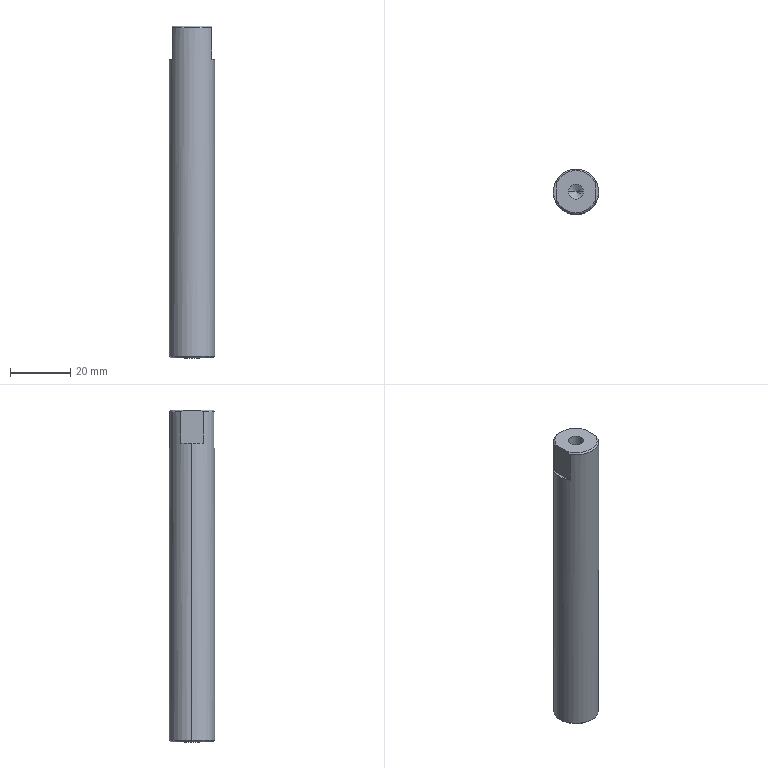Part | SolidWorks | features HoleWzd 2, BaseBody 1 | 1 solid | 20 faces | box 15 x 15 x 110 mm | volume 18709 mm3 | cone 8 | cylinder 6 | plane 6 | commonest cylinder face diameters 5 x4 15 x2
STEP:
#1=CARTESIAN_POINT('',(2.5,0.,-95.));
#2=VERTEX_POINT('',#1);
#3=CARTESIAN_POINT('',(-2.5,0.,-95.));
#4=VERTEX_POINT('',#3);
#5=CARTESIAN_POINT('',(0.,0.,-95.));
#6=DIRECTION('',(0.,0.,-1.));
#7=DIRECTION('',(-1.,0.,0.));
#8=AXIS2_PLACEMENT_3D('',#5,#6,#7);
#9=CIRCLE('',#8,2.5);
#10=EDGE_CURVE('',#2,#4,#9,.T.);
#11=ORIENTED_EDGE('',*,*,#10,.F.);
#12=CARTESIAN_POINT('',(2.5,0.,-110.));
#13=VERTEX_POINT('',#12);
#14=CARTESIAN_POINT('',(2.5,0.,-110.));
#15=DIRECTION('',(0.,0.,-1.));
#16=VECTOR('',#15,1000.);
#17=LINE('',#14,#16);
#18=EDGE_CURVE('',#2,#13,#17,.T.);
#19=ORIENTED_EDGE('',*,*,#18,.T.);
#20=CARTESIAN_POINT('',(-2.5,0.,-110.));
#21=VERTEX_POINT('',#20);
#22=CARTESIAN_POINT('',(0.,0.,-110.));
#23=DIRECTION('',(0.,0.,-1.));
#24=DIRECTION('',(-1.,0.,0.));
#25=AXIS2_PLACEMENT_3D('',#22,#23,#24);
#26=CIRCLE('',#25,2.5);
#27=EDGE_CURVE('',#13,#21,#26,.T.);
#28=ORIENTED_EDGE('',*,*,#27,.T.);
#29=CARTESIAN_POINT('',(-2.5,0.,-110.));
#30=DIRECTION('',(0.,0.,-1.));
#31=VECTOR('',#30,1000.);
#32=LINE('',#29,#31);
#33=EDGE_CURVE('',#4,#21,#32,.T.);
#34=ORIENTED_EDGE('',*,*,#33,.F.);
#35=EDGE_LOOP('',(#11,#19,#28,#34));
#36=FACE_OUTER_BOUND('',#35,.T.);
#37=CARTESIAN_POINT('',(0.,0.,-110.));
#38=DIRECTION('',(0.,0.,-1.));
#39=DIRECTION('',(-1.,0.,0.));
#40=AXIS2_PLACEMENT_3D('',#37,#38,#39);
#41=CYLINDRICAL_SURFACE('',#40,2.5);
#42=ADVANCED_FACE('',(#36),#41,.F.);
#43=CARTESIAN_POINT('',(0.,0.,-93.498));
#44=VERTEX_POINT('',#43);
#45=CARTESIAN_POINT('',(-2.5,0.,-95.));
#46=DIRECTION('',(-0.8572,0.,-0.515));
#47=VECTOR('',#46,1000.);
#48=LINE('',#45,#47);
#49=EDGE_CURVE('',#44,#4,#48,.T.);
#50=ORIENTED_EDGE('',*,*,#49,.F.);
#51=CARTESIAN_POINT('',(2.5,0.,-95.));
#52=DIRECTION('',(0.8572,0.,-0.515));
#53=VECTOR('',#52,1000.);
#54=LINE('',#51,#53);
#55=EDGE_CURVE('',#44,#2,#54,.T.);
#56=ORIENTED_EDGE('',*,*,#55,.T.);
#57=ORIENTED_EDGE('',*,*,#10,.T.);
#58=EDGE_LOOP('',(#50,#56,#57));
#59=FACE_OUTER_BOUND('',#58,.T.);
#60=CARTESIAN_POINT('',(0.,0.,-95.));
#61=DIRECTION('',(0.,0.,-1.));
#62=DIRECTION('',(-1.,0.,0.));
#63=AXIS2_PLACEMENT_3D('',#60,#61,#62);
#64=CONICAL_SURFACE('',#63,2.5,1.03);
#65=ADVANCED_FACE('',(#59),#64,.F.);
#66=CARTESIAN_POINT('',(-2.5,0.,-15.));
#67=VERTEX_POINT('',#66);
#68=CARTESIAN_POINT('',(2.5,0.,-15.));
#69=VERTEX_POINT('',#68);
#70=CARTESIAN_POINT('',(0.,0.,-15.));
#71=DIRECTION('',(0.,0.,1.));
#72=DIRECTION('',(1.,0.,0.));
#73=AXIS2_PLACEMENT_3D('',#70,#71,#72);
#74=CIRCLE('',#73,2.5);
#75=EDGE_CURVE('',#67,#69,#74,.T.);
#76=ORIENTED_EDGE('',*,*,#75,.F.);
#77=CARTESIAN_POINT('',(-2.5,0.,0.));
#78=VERTEX_POINT('',#77);
#79=CARTESIAN_POINT('',(-2.5,0.,0.));
#80=DIRECTION('',(0.,0.,1.));
#81=VECTOR('',#80,1000.);
#82=LINE('',#79,#81);
#83=EDGE_CURVE('',#67,#78,#82,.T.);
#84=ORIENTED_EDGE('',*,*,#83,.T.);
#85=CARTESIAN_POINT('',(2.5,0.,0.));
#86=VERTEX_POINT('',#85);
#87=CARTESIAN_POINT('',(0.,0.,0.));
#88=DIRECTION('',(0.,0.,1.));
#89=DIRECTION('',(1.,0.,0.));
#90=AXIS2_PLACEMENT_3D('',#87,#88,#89);
#91=CIRCLE('',#90,2.5);
#92=EDGE_CURVE('',#78,#86,#91,.T.);
#93=ORIENTED_EDGE('',*,*,#92,.T.);
#94=CARTESIAN_POINT('',(2.5,0.,0.));
#95=DIRECTION('',(0.,0.,1.));
#96=VECTOR('',#95,1000.);
#97=LINE('',#94,#96);
#98=EDGE_CURVE('',#69,#86,#97,.T.);
#99=ORIENTED_EDGE('',*,*,#98,.F.);
#100=EDGE_LOOP('',(#76,#84,#93,#99));
#101=FACE_OUTER_BOUND('',#100,.T.);
#102=CARTESIAN_POINT('',(0.,0.,0.));
#103=DIRECTION('',(0.,0.,1.));
#104=DIRECTION('',(1.,0.,0.));
#105=AXIS2_PLACEMENT_3D('',#102,#103,#104);
#106=CYLINDRICAL_SURFACE('',#105,2.5);
#107=ADVANCED_FACE('',(#101),#106,.F.);
#108=CARTESIAN_POINT('',(0.,0.,-16.502));
#109=VERTEX_POINT('',#108);
#110=CARTESIAN_POINT('',(2.5,0.,-15.));
#111=DIRECTION('',(0.8572,0.,0.515));
#112=VECTOR('',#111,1000.);
#113=LINE('',#110,#112);
#114=EDGE_CURVE('',#109,#69,#113,.T.);
#115=ORIENTED_EDGE('',*,*,#114,.F.);
#116=CARTESIAN_POINT('',(-2.5,0.,-15.));
#117=DIRECTION('',(-0.8572,0.,0.515));
#118=VECTOR('',#117,1000.);
#119=LINE('',#116,#118);
#120=EDGE_CURVE('',#109,#67,#119,.T.);
#121=ORIENTED_EDGE('',*,*,#120,.T.);
#122=ORIENTED_EDGE('',*,*,#75,.T.);
#123=EDGE_LOOP('',(#115,#121,#122));
#124=FACE_OUTER_BOUND('',#123,.T.);
#125=CARTESIAN_POINT('',(0.,0.,-15.));
#126=DIRECTION('',(0.,0.,1.));
#127=DIRECTION('',(1.,0.,0.));
#128=AXIS2_PLACEMENT_3D('',#125,#126,#127);
#129=CONICAL_SURFACE('',#128,2.5,1.03);
#130=ADVANCED_FACE('',(#124),#129,.F.);
#131=CARTESIAN_POINT('',(0.,7.5,-109.5));
#132=VERTEX_POINT('',#131);
#133=CARTESIAN_POINT('',(-7.5,0.,-109.5));
#134=VERTEX_POINT('',#133);
#135=CARTESIAN_POINT('',(0.,0.,-109.5));
#136=DIRECTION('',(0.,0.,1.));
#137=DIRECTION('',(1.,0.,0.));
#138=AXIS2_PLACEMENT_3D('',#135,#136,#137);
#139=CIRCLE('',#138,7.5);
#140=EDGE_CURVE('',#132,#134,#139,.T.);
#141=ORIENTED_EDGE('',*,*,#140,.T.);
#142=CARTESIAN_POINT('',(-7.5,0.,-11.));
#143=VERTEX_POINT('',#142);
#144=CARTESIAN_POINT('',(-7.5,0.,-110.));
#145=DIRECTION('',(0.,0.,1.));
#146=VECTOR('',#145,1000.);
#147=LINE('',#144,#146);
#148=EDGE_CURVE('',#134,#143,#147,.T.);
#149=ORIENTED_EDGE('',*,*,#148,.T.);
#150=CARTESIAN_POINT('',(-6.5,3.742,-11.));
#151=VERTEX_POINT('',#150);
#152=CARTESIAN_POINT('',(0.,0.,-11.));
#153=DIRECTION('',(0.,0.,-1.));
#154=DIRECTION('',(1.,0.,0.));
#155=AXIS2_PLACEMENT_3D('',#152,#153,#154);
#156=CIRCLE('',#155,7.5);
#157=EDGE_CURVE('',#143,#151,#156,.T.);
#158=ORIENTED_EDGE('',*,*,#157,.T.);
#159=CARTESIAN_POINT('',(-6.5,3.742,-0.5));
#160=VERTEX_POINT('',#159);
#161=CARTESIAN_POINT('',(-6.5,3.742,-110.));
#162=DIRECTION('',(0.,0.,1.));
#163=VECTOR('',#162,1000.);
#164=LINE('',#161,#163);
#165=EDGE_CURVE('',#151,#160,#164,.T.);
#166=ORIENTED_EDGE('',*,*,#165,.T.);
#167=CARTESIAN_POINT('',(6.5,3.742,-0.5));
#168=VERTEX_POINT('',#167);
#169=CARTESIAN_POINT('',(0.,0.,-0.5));
#170=DIRECTION('',(0.,0.,-1.));
#171=DIRECTION('',(1.,0.,0.));
#172=AXIS2_PLACEMENT_3D('',#169,#170,#171);
#173=CIRCLE('',#172,7.5);
#174=EDGE_CURVE('',#160,#168,#173,.T.);
#175=ORIENTED_EDGE('',*,*,#174,.T.);
#176=CARTESIAN_POINT('',(6.5,3.742,-11.));
#177=VERTEX_POINT('',#176);
#178=CARTESIAN_POINT('',(6.5,3.742,-110.));
#179=DIRECTION('',(0.,0.,-1.));
#180=VECTOR('',#179,1000.);
#181=LINE('',#178,#180);
#182=EDGE_CURVE('',#168,#177,#181,.T.);
#183=ORIENTED_EDGE('',*,*,#182,.T.);
#184=CARTESIAN_POINT('',(7.5,0.,-11.));
#185=VERTEX_POINT('',#184);
#186=CARTESIAN_POINT('',(0.,0.,-11.));
#187=DIRECTION('',(0.,0.,-1.));
#188=DIRECTION('',(1.,0.,0.));
#189=AXIS2_PLACEMENT_3D('',#186,#187,#188);
#190=CIRCLE('',#189,7.5);
#191=EDGE_CURVE('',#177,#185,#190,.T.);
#192=ORIENTED_EDGE('',*,*,#191,.T.);
#193=CARTESIAN_POINT('',(7.5,0.,-109.5));
#194=VERTEX_POINT('',#193);
#195=CARTESIAN_POINT('',(7.5,0.,-110.));
#196=DIRECTION('',(0.,0.,1.));
#197=VECTOR('',#196,1000.);
#198=LINE('',#195,#197);
#199=EDGE_CURVE('',#194,#185,#198,.T.);
#200=ORIENTED_EDGE('',*,*,#199,.F.);
#201=CARTESIAN_POINT('',(0.,0.,-109.5));
#202=DIRECTION('',(0.,0.,1.));
#203=DIRECTION('',(1.,0.,0.));
#204=AXIS2_PLACEMENT_3D('',#201,#202,#203);
#205=CIRCLE('',#204,7.5);
#206=EDGE_CURVE('',#194,#132,#205,.T.);
#207=ORIENTED_EDGE('',*,*,#206,.T.);
#208=EDGE_LOOP('',(#141,#149,#158,#166,#175,#183,#192,#200,#207));
#209=FACE_OUTER_BOUND('',#208,.T.);
#210=CARTESIAN_POINT('',(0.,0.,-110.));
#211=DIRECTION('',(0.,0.,1.));
#212=DIRECTION('',(1.,0.,0.));
#213=AXIS2_PLACEMENT_3D('',#210,#211,#212);
#214=CYLINDRICAL_SURFACE('',#213,7.5);
#215=ADVANCED_FACE('',(#209),#214,.T.);
#216=CARTESIAN_POINT('',(0.,-7.,-110.));
#217=VERTEX_POINT('',#216);
#218=CARTESIAN_POINT('',(0.,7.,-110.));
#219=VERTEX_POINT('',#218);
#220=CARTESIAN_POINT('',(0.,0.,-110.));
#221=DIRECTION('',(0.,0.,1.));
#222=DIRECTION('',(0.,-1.,0.));
#223=AXIS2_PLACEMENT_3D('',#220,#221,#222);
#224=CIRCLE('',#223,7.);
#225=EDGE_CURVE('',#217,#219,#224,.T.);
#226=ORIENTED_EDGE('',*,*,#225,.T.);
#227=CARTESIAN_POINT('',(0.,7.5,-109.5));
#228=DIRECTION('',(0.,0.7071,0.7071));
#229=VECTOR('',#228,1000.);
#230=LINE('',#227,#229);
#231=EDGE_CURVE('',#219,#132,#230,.T.);
#232=ORIENTED_EDGE('',*,*,#231,.T.);
#233=ORIENTED_EDGE('',*,*,#206,.F.);
#234=CARTESIAN_POINT('',(0.,-7.5,-109.5));
#235=VERTEX_POINT('',#234);
#236=CARTESIAN_POINT('',(0.,0.,-109.5));
#237=DIRECTION('',(0.,0.,1.));
#238=DIRECTION('',(1.,0.,0.));
#239=AXIS2_PLACEMENT_3D('',#236,#237,#238);
#240=CIRCLE('',#239,7.5);
#241=EDGE_CURVE('',#235,#194,#240,.T.);
#242=ORIENTED_EDGE('',*,*,#241,.F.);
#243=CARTESIAN_POINT('',(0.,-7.5,-109.5));
#244=DIRECTION('',(0.,-0.7071,0.7071));
#245=VECTOR('',#244,1000.);
#246=LINE('',#243,#245);
#247=EDGE_CURVE('',#217,#235,#246,.T.);
#248=ORIENTED_EDGE('',*,*,#247,.F.);
#249=EDGE_LOOP('',(#226,#232,#233,#242,#248));
#250=FACE_OUTER_BOUND('',#249,.T.);
#251=CARTESIAN_POINT('',(0.,0.,-109.5));
#252=DIRECTION('',(0.,0.,1.));
#253=DIRECTION('',(0.,-1.,0.));
#254=AXIS2_PLACEMENT_3D('',#251,#252,#253);
#255=CONICAL_SURFACE('',#254,7.5,0.7854);
#256=ADVANCED_FACE('',(#250),#255,.T.);
#257=ORIENTED_EDGE('',*,*,#148,.F.);
#258=CARTESIAN_POINT('',(0.,0.,-109.5));
#259=DIRECTION('',(0.,0.,1.));
#260=DIRECTION('',(1.,0.,0.));
#261=AXIS2_PLACEMENT_3D('',#258,#259,#260);
#262=CIRCLE('',#261,7.5);
#263=EDGE_CURVE('',#134,#235,#262,.T.);
#264=ORIENTED_EDGE('',*,*,#263,.T.);
#265=ORIENTED_EDGE('',*,*,#241,.T.);
#266=ORIENTED_EDGE('',*,*,#199,.T.);
#267=CARTESIAN_POINT('',(6.5,-3.742,-11.));
#268=VERTEX_POINT('',#267);
#269=CARTESIAN_POINT('',(0.,0.,-11.));
#270=DIRECTION('',(0.,0.,-1.));
#271=DIRECTION('',(1.,0.,0.));
#272=AXIS2_PLACEMENT_3D('',#269,#270,#271);
#273=CIRCLE('',#272,7.5);
#274=EDGE_CURVE('',#185,#268,#273,.T.);
#275=ORIENTED_EDGE('',*,*,#274,.T.);
#276=CARTESIAN_POINT('',(6.5,-3.742,-0.5));
#277=VERTEX_POINT('',#276);
#278=CARTESIAN_POINT('',(6.5,-3.742,-110.));
#279=DIRECTION('',(0.,0.,1.));
#280=VECTOR('',#279,1000.);
#281=LINE('',#278,#280);
#282=EDGE_CURVE('',#268,#277,#281,.T.);
#283=ORIENTED_EDGE('',*,*,#282,.T.);
#284=CARTESIAN_POINT('',(-6.5,-3.742,-0.5));
#285=VERTEX_POINT('',#284);
#286=CARTESIAN_POINT('',(0.,0.,-0.5));
#287=DIRECTION('',(0.,0.,-1.));
#288=DIRECTION('',(1.,0.,0.));
#289=AXIS2_PLACEMENT_3D('',#286,#287,#288);
#290=CIRCLE('',#289,7.5);
#291=EDGE_CURVE('',#277,#285,#290,.T.);
#292=ORIENTED_EDGE('',*,*,#291,.T.);
#293=CARTESIAN_POINT('',(-6.5,-3.742,-11.));
#294=VERTEX_POINT('',#293);
#295=CARTESIAN_POINT('',(-6.5,-3.742,-110.));
#296=DIRECTION('',(0.,0.,-1.));
#297=VECTOR('',#296,1000.);
#298=LINE('',#295,#297);
#299=EDGE_CURVE('',#285,#294,#298,.T.);
#300=ORIENTED_EDGE('',*,*,#299,.T.);
#301=CARTESIAN_POINT('',(0.,0.,-11.));
#302=DIRECTION('',(0.,0.,-1.));
#303=DIRECTION('',(1.,0.,0.));
#304=AXIS2_PLACEMENT_3D('',#301,#302,#303);
#305=CIRCLE('',#304,7.5);
#306=EDGE_CURVE('',#294,#143,#305,.T.);
#307=ORIENTED_EDGE('',*,*,#306,.T.);
#308=EDGE_LOOP('',(#257,#264,#265,#266,#275,#283,#292,#300,#307));
#309=FACE_OUTER_BOUND('',#308,.T.);
#310=CARTESIAN_POINT('',(0.,0.,-110.));
#311=DIRECTION('',(0.,0.,1.));
#312=DIRECTION('',(1.,0.,0.));
#313=AXIS2_PLACEMENT_3D('',#310,#311,#312);
#314=CYLINDRICAL_SURFACE('',#313,7.5);
#315=ADVANCED_FACE('',(#309),#314,.T.);
#316=ORIENTED_EDGE('',*,*,#306,.F.);
#317=CARTESIAN_POINT('',(-6.5,0.,-11.));
#318=DIRECTION('',(0.,1.,0.));
#319=VECTOR('',#318,1000.);
#320=LINE('',#317,#319);
#321=EDGE_CURVE('',#294,#151,#320,.T.);
#322=ORIENTED_EDGE('',*,*,#321,.T.);
#323=ORIENTED_EDGE('',*,*,#157,.F.);
#324=EDGE_LOOP('',(#316,#322,#323));
#325=FACE_OUTER_BOUND('',#324,.T.);
#326=CARTESIAN_POINT('',(0.,0.,-11.));
#327=DIRECTION('',(0.,0.,1.));
#328=DIRECTION('',(1.,0.,0.));
#329=AXIS2_PLACEMENT_3D('',#326,#327,#328);
#330=PLANE('',#329);
#331=ADVANCED_FACE('',(#325),#330,.T.);
#332=ORIENTED_EDGE('',*,*,#321,.F.);
#333=ORIENTED_EDGE('',*,*,#299,.F.);
#334=CARTESIAN_POINT('',(-6.5,-2.598,0.));
#335=VERTEX_POINT('',#334);
#336=CARTESIAN_POINT('',(-6.5,-3.742,-0.5));
#337=CARTESIAN_POINT('',(-6.5,-3.369,-0.314));
#338=CARTESIAN_POINT('',(-6.5,-2.989,-0.145));
#339=CARTESIAN_POINT('',(-6.5,-2.598,0.));
#340=B_SPLINE_CURVE_WITH_KNOTS('',3,(#336,#337,#338,#339),.UNSPECIFIED.,.F.,.F.,(4,4),(0.,0.001248),.UNSPECIFIED.);
#341=EDGE_CURVE('',#285,#335,#340,.T.);
#342=ORIENTED_EDGE('',*,*,#341,.T.);
#343=CARTESIAN_POINT('',(-6.5,2.598,0.));
#344=VERTEX_POINT('',#343);
#345=CARTESIAN_POINT('',(-6.5,3.742,0.));
#346=DIRECTION('',(0.,1.,0.));
#347=VECTOR('',#346,1000.);
#348=LINE('',#345,#347);
#349=EDGE_CURVE('',#335,#344,#348,.T.);
#350=ORIENTED_EDGE('',*,*,#349,.T.);
#351=CARTESIAN_POINT('',(-6.5,2.598,0.));
#352=CARTESIAN_POINT('',(-6.5,2.989,-0.145));
#353=CARTESIAN_POINT('',(-6.5,3.369,-0.314));
#354=CARTESIAN_POINT('',(-6.5,3.742,-0.5));
#355=B_SPLINE_CURVE_WITH_KNOTS('',3,(#351,#352,#353,#354),.UNSPECIFIED.,.F.,.F.,(4,4),(0.,0.001248),.UNSPECIFIED.);
#356=EDGE_CURVE('',#344,#160,#355,.T.);
#357=ORIENTED_EDGE('',*,*,#356,.T.);
#358=ORIENTED_EDGE('',*,*,#165,.F.);
#359=EDGE_LOOP('',(#332,#333,#342,#350,#357,#358));
#360=FACE_OUTER_BOUND('',#359,.T.);
#361=CARTESIAN_POINT('',(-6.5,3.742,-11.));
#362=DIRECTION('',(-1.,0.,0.));
#363=DIRECTION('',(0.,0.,1.));
#364=AXIS2_PLACEMENT_3D('',#361,#362,#363);
#365=PLANE('',#364);
#366=ADVANCED_FACE('',(#360),#365,.T.);
#367=ORIENTED_EDGE('',*,*,#341,.F.);
#368=ORIENTED_EDGE('',*,*,#291,.F.);
#369=CARTESIAN_POINT('',(6.5,-2.598,0.));
#370=VERTEX_POINT('',#369);
#371=CARTESIAN_POINT('',(6.5,-3.742,-0.5));
#372=CARTESIAN_POINT('',(6.5,-3.369,-0.314));
#373=CARTESIAN_POINT('',(6.5,-2.989,-0.145));
#374=CARTESIAN_POINT('',(6.5,-2.598,0.));
#375=B_SPLINE_CURVE_WITH_KNOTS('',3,(#371,#372,#373,#374),.UNSPECIFIED.,.F.,.F.,(4,4),(0.,0.001248),.UNSPECIFIED.);
#376=EDGE_CURVE('',#277,#370,#375,.T.);
#377=ORIENTED_EDGE('',*,*,#376,.T.);
#378=CARTESIAN_POINT('',(0.,0.,0.));
#379=DIRECTION('',(0.,0.,-1.));
#380=DIRECTION('',(0.,1.,0.));
#381=AXIS2_PLACEMENT_3D('',#378,#379,#380);
#382=CIRCLE('',#381,7.);
#383=EDGE_CURVE('',#370,#335,#382,.T.);
#384=ORIENTED_EDGE('',*,*,#383,.T.);
#385=EDGE_LOOP('',(#367,#368,#377,#384));
#386=FACE_OUTER_BOUND('',#385,.T.);
#387=CARTESIAN_POINT('',(0.,0.,-0.5));
#388=DIRECTION('',(0.,0.,-1.));
#389=DIRECTION('',(0.,1.,0.));
#390=AXIS2_PLACEMENT_3D('',#387,#388,#389);
#391=CONICAL_SURFACE('',#390,7.5,0.7854);
#392=ADVANCED_FACE('',(#386),#391,.T.);
#393=CARTESIAN_POINT('',(6.5,-3.742,-11.));
#394=DIRECTION('',(0.,1.,0.));
#395=VECTOR('',#394,1000.);
#396=LINE('',#393,#395);
#397=EDGE_CURVE('',#268,#177,#396,.T.);
#398=ORIENTED_EDGE('',*,*,#397,.T.);
#399=ORIENTED_EDGE('',*,*,#182,.F.);
#400=CARTESIAN_POINT('',(6.5,2.598,0.));
#401=VERTEX_POINT('',#400);
#402=CARTESIAN_POINT('',(6.5,3.742,-0.5));
#403=CARTESIAN_POINT('',(6.5,3.369,-0.314));
#404=CARTESIAN_POINT('',(6.5,2.989,-0.145));
#405=CARTESIAN_POINT('',(6.5,2.598,0.));
#406=B_SPLINE_CURVE_WITH_KNOTS('',3,(#402,#403,#404,#405),.UNSPECIFIED.,.F.,.F.,(4,4),(0.,0.001248),.UNSPECIFIED.);
#407=EDGE_CURVE('',#168,#401,#406,.T.);
#408=ORIENTED_EDGE('',*,*,#407,.T.);
#409=CARTESIAN_POINT('',(6.5,-3.742,0.));
#410=DIRECTION('',(0.,-1.,0.));
#411=VECTOR('',#410,1000.);
#412=LINE('',#409,#411);
#413=EDGE_CURVE('',#401,#370,#412,.T.);
#414=ORIENTED_EDGE('',*,*,#413,.T.);
#415=ORIENTED_EDGE('',*,*,#376,.F.);
#416=ORIENTED_EDGE('',*,*,#282,.F.);
#417=EDGE_LOOP('',(#398,#399,#408,#414,#415,#416));
#418=FACE_OUTER_BOUND('',#417,.T.);
#419=CARTESIAN_POINT('',(6.5,-3.742,-11.));
#420=DIRECTION('',(1.,0.,0.));
#421=DIRECTION('',(0.,0.,-1.));
#422=AXIS2_PLACEMENT_3D('',#419,#420,#421);
#423=PLANE('',#422);
#424=ADVANCED_FACE('',(#418),#423,.T.);
#425=ORIENTED_EDGE('',*,*,#191,.F.);
#426=ORIENTED_EDGE('',*,*,#397,.F.);
#427=ORIENTED_EDGE('',*,*,#274,.F.);
#428=EDGE_LOOP('',(#425,#426,#427));
#429=FACE_OUTER_BOUND('',#428,.T.);
#430=CARTESIAN_POINT('',(0.,0.,-11.));
#431=DIRECTION('',(0.,0.,1.));
#432=DIRECTION('',(1.,0.,0.));
#433=AXIS2_PLACEMENT_3D('',#430,#431,#432);
#434=PLANE('',#433);
#435=ADVANCED_FACE('',(#429),#434,.T.);
#436=ORIENTED_EDGE('',*,*,#407,.F.);
#437=ORIENTED_EDGE('',*,*,#174,.F.);
#438=ORIENTED_EDGE('',*,*,#356,.F.);
#439=CARTESIAN_POINT('',(0.,0.,0.));
#440=DIRECTION('',(0.,0.,-1.));
#441=DIRECTION('',(-1.,0.,0.));
#442=AXIS2_PLACEMENT_3D('',#439,#440,#441);
#443=CIRCLE('',#442,7.);
#444=EDGE_CURVE('',#344,#401,#443,.T.);
#445=ORIENTED_EDGE('',*,*,#444,.T.);
#446=EDGE_LOOP('',(#436,#437,#438,#445));
#447=FACE_OUTER_BOUND('',#446,.T.);
#448=CARTESIAN_POINT('',(0.,0.,-0.5));
#449=DIRECTION('',(0.,0.,-1.));
#450=DIRECTION('',(-1.,0.,0.));
#451=AXIS2_PLACEMENT_3D('',#448,#449,#450);
#452=CONICAL_SURFACE('',#451,7.5,0.7854);
#453=ADVANCED_FACE('',(#447),#452,.T.);
#454=ORIENTED_EDGE('',*,*,#231,.F.);
#455=CARTESIAN_POINT('',(0.,0.,-110.));
#456=DIRECTION('',(0.,0.,1.));
#457=DIRECTION('',(0.,-1.,0.));
#458=AXIS2_PLACEMENT_3D('',#455,#456,#457);
#459=CIRCLE('',#458,7.);
#460=EDGE_CURVE('',#219,#217,#459,.T.);
#461=ORIENTED_EDGE('',*,*,#460,.T.);
#462=ORIENTED_EDGE('',*,*,#247,.T.);
#463=ORIENTED_EDGE('',*,*,#263,.F.);
#464=ORIENTED_EDGE('',*,*,#140,.F.);
#465=EDGE_LOOP('',(#454,#461,#462,#463,#464));
#466=FACE_OUTER_BOUND('',#465,.T.);
#467=CARTESIAN_POINT('',(0.,0.,-109.5));
#468=DIRECTION('',(0.,0.,1.));
#469=DIRECTION('',(0.,-1.,0.));
#470=AXIS2_PLACEMENT_3D('',#467,#468,#469);
#471=CONICAL_SURFACE('',#470,7.5,0.7854);
#472=ADVANCED_FACE('',(#466),#471,.T.);
#473=CARTESIAN_POINT('',(0.,0.,0.));
#474=DIRECTION('',(0.,0.,1.));
#475=DIRECTION('',(1.,0.,0.));
#476=AXIS2_PLACEMENT_3D('',#473,#474,#475);
#477=CIRCLE('',#476,2.5);
#478=EDGE_CURVE('',#86,#78,#477,.T.);
#479=ORIENTED_EDGE('',*,*,#478,.F.);
#480=ORIENTED_EDGE('',*,*,#92,.F.);
#481=EDGE_LOOP('',(#479,#480));
#482=FACE_BOUND('',#481,.T.);
#483=ORIENTED_EDGE('',*,*,#349,.F.);
#484=ORIENTED_EDGE('',*,*,#383,.F.);
#485=ORIENTED_EDGE('',*,*,#413,.F.);
#486=ORIENTED_EDGE('',*,*,#444,.F.);
#487=EDGE_LOOP('',(#483,#484,#485,#486));
#488=FACE_OUTER_BOUND('',#487,.T.);
#489=CARTESIAN_POINT('',(0.,0.,0.));
#490=DIRECTION('',(0.,0.,-1.));
#491=DIRECTION('',(-1.,0.,0.));
#492=AXIS2_PLACEMENT_3D('',#489,#490,#491);
#493=PLANE('',#492);
#494=ADVANCED_FACE('',(#482,#488),#493,.F.);
#495=ORIENTED_EDGE('',*,*,#225,.F.);
#496=ORIENTED_EDGE('',*,*,#460,.F.);
#497=EDGE_LOOP('',(#495,#496));
#498=FACE_OUTER_BOUND('',#497,.T.);
#499=CARTESIAN_POINT('',(0.,0.,-110.));
#500=DIRECTION('',(0.,0.,-1.));
#501=DIRECTION('',(-1.,0.,0.));
#502=AXIS2_PLACEMENT_3D('',#499,#500,#501);
#503=CIRCLE('',#502,2.5);
#504=EDGE_CURVE('',#21,#13,#503,.T.);
#505=ORIENTED_EDGE('',*,*,#504,.F.);
#506=ORIENTED_EDGE('',*,*,#27,.F.);
#507=EDGE_LOOP('',(#505,#506));
#508=FACE_BOUND('',#507,.T.);
#509=CARTESIAN_POINT('',(0.,7.,-110.));
#510=DIRECTION('',(0.,0.,1.));
#511=DIRECTION('',(1.,0.,0.));
#512=AXIS2_PLACEMENT_3D('',#509,#510,#511);
#513=PLANE('',#512);
#514=ADVANCED_FACE('',(#498,#508),#513,.F.);
#515=ORIENTED_EDGE('',*,*,#120,.F.);
#516=ORIENTED_EDGE('',*,*,#114,.T.);
#517=CARTESIAN_POINT('',(0.,0.,-15.));
#518=DIRECTION('',(0.,0.,1.));
#519=DIRECTION('',(1.,0.,0.));
#520=AXIS2_PLACEMENT_3D('',#517,#518,#519);
#521=CIRCLE('',#520,2.5);
#522=EDGE_CURVE('',#69,#67,#521,.T.);
#523=ORIENTED_EDGE('',*,*,#522,.T.);
#524=EDGE_LOOP('',(#515,#516,#523));
#525=FACE_OUTER_BOUND('',#524,.T.);
#526=CARTESIAN_POINT('',(0.,0.,-15.));
#527=DIRECTION('',(0.,0.,1.));
#528=DIRECTION('',(1.,0.,0.));
#529=AXIS2_PLACEMENT_3D('',#526,#527,#528);
#530=CONICAL_SURFACE('',#529,2.5,1.03);
#531=ADVANCED_FACE('',(#525),#530,.F.);
#532=ORIENTED_EDGE('',*,*,#83,.F.);
#533=ORIENTED_EDGE('',*,*,#522,.F.);
#534=ORIENTED_EDGE('',*,*,#98,.T.);
#535=ORIENTED_EDGE('',*,*,#478,.T.);
#536=EDGE_LOOP('',(#532,#533,#534,#535));
#537=FACE_OUTER_BOUND('',#536,.T.);
#538=CARTESIAN_POINT('',(0.,0.,0.));
#539=DIRECTION('',(0.,0.,1.));
#540=DIRECTION('',(1.,0.,0.));
#541=AXIS2_PLACEMENT_3D('',#538,#539,#540);
#542=CYLINDRICAL_SURFACE('',#541,2.5);
#543=ADVANCED_FACE('',(#537),#542,.F.);
#544=ORIENTED_EDGE('',*,*,#55,.F.);
#545=ORIENTED_EDGE('',*,*,#49,.T.);
#546=CARTESIAN_POINT('',(0.,0.,-95.));
#547=DIRECTION('',(0.,0.,-1.));
#548=DIRECTION('',(-1.,0.,0.));
#549=AXIS2_PLACEMENT_3D('',#546,#547,#548);
#550=CIRCLE('',#549,2.5);
#551=EDGE_CURVE('',#4,#2,#550,.T.);
#552=ORIENTED_EDGE('',*,*,#551,.T.);
#553=EDGE_LOOP('',(#544,#545,#552));
#554=FACE_OUTER_BOUND('',#553,.T.);
#555=CARTESIAN_POINT('',(0.,0.,-95.));
#556=DIRECTION('',(0.,0.,-1.));
#557=DIRECTION('',(-1.,0.,0.));
#558=AXIS2_PLACEMENT_3D('',#555,#556,#557);
#559=CONICAL_SURFACE('',#558,2.5,1.03);
#560=ADVANCED_FACE('',(#554),#559,.F.);
#561=ORIENTED_EDGE('',*,*,#18,.F.);
#562=ORIENTED_EDGE('',*,*,#551,.F.);
#563=ORIENTED_EDGE('',*,*,#33,.T.);
#564=ORIENTED_EDGE('',*,*,#504,.T.);
#565=EDGE_LOOP('',(#561,#562,#563,#564));
#566=FACE_OUTER_BOUND('',#565,.T.);
#567=CARTESIAN_POINT('',(0.,0.,-110.));
#568=DIRECTION('',(0.,0.,-1.));
#569=DIRECTION('',(-1.,0.,0.));
#570=AXIS2_PLACEMENT_3D('',#567,#568,#569);
#571=CYLINDRICAL_SURFACE('',#570,2.5);
#572=ADVANCED_FACE('',(#566),#571,.F.);
#573=CLOSED_SHELL('',(#42,#65,#107,#130,#215,#256,#315,#331,#366,#392,#424,#435,#453,#472,#494,#514,#531,#543,#560,#572));
#574=MANIFOLD_SOLID_BREP('',#573);
#575=CARTESIAN_POINT('',(0.,0.,0.));
#576=DIRECTION('',(0.,0.,1.));
#577=DIRECTION('',(1.,0.,0.));
#578=AXIS2_PLACEMENT_3D('',#575,#576,#577);
#579=(LENGTH_UNIT()NAMED_UNIT(*)SI_UNIT(.MILLI.,.METRE.));
#580=UNCERTAINTY_MEASURE_WITH_UNIT(LENGTH_MEASURE(0.00001),#579,'','');
#581=(NAMED_UNIT(*)PLANE_ANGLE_UNIT()SI_UNIT($,.RADIAN.));
#582=(NAMED_UNIT(*)SI_UNIT($,.STERADIAN.)SOLID_ANGLE_UNIT());
#583=(GEOMETRIC_REPRESENTATION_CONTEXT(3)GLOBAL_UNCERTAINTY_ASSIGNED_CONTEXT((#580))GLOBAL_UNIT_ASSIGNED_CONTEXT((#579,#581,#582))REPRESENTATION_CONTEXT('',''));
#584=ADVANCED_BREP_SHAPE_REPRESENTATION('',(#574,#578),#583);